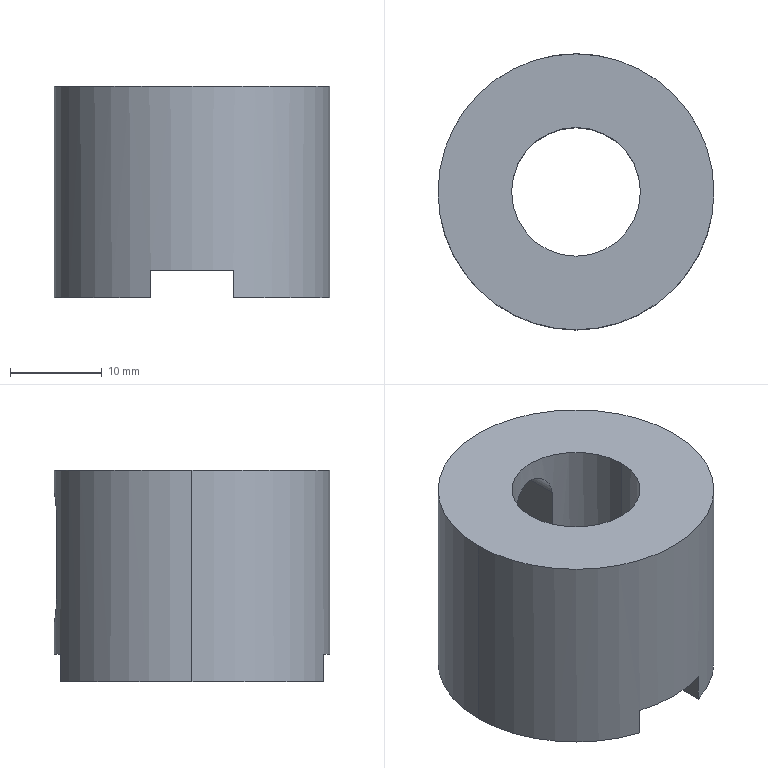Part | STEP file | BU-E01#130 | 1 solid | 18 faces | box 30 x 30 x 23 mm | volume 11677 mm3 | plane 11 | cylinder 7 | commonest cylinder face diameters 5.5 x3 14 x2 30 x2